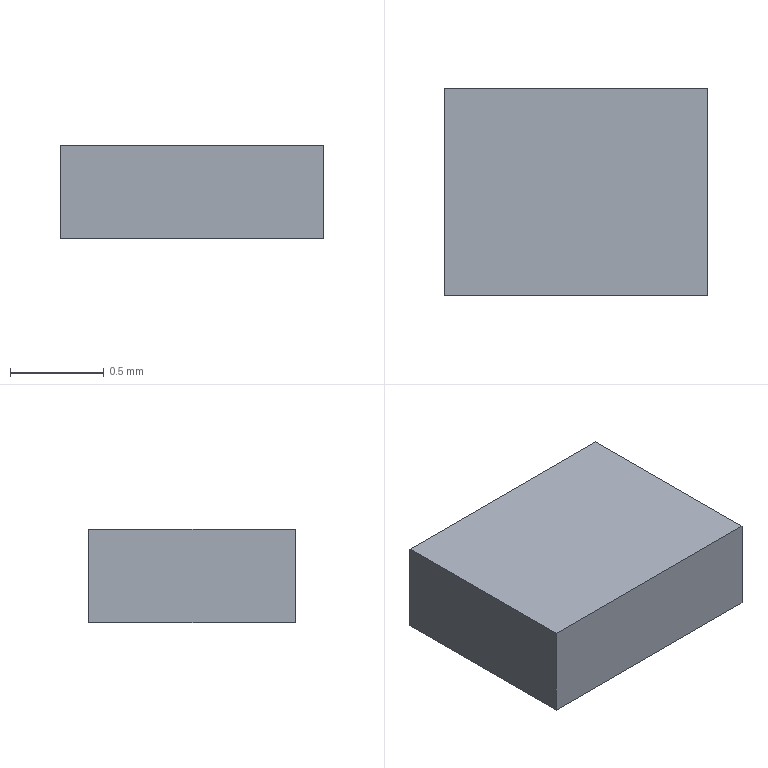Part | Creo | 1 solid | 6 faces | box 1.4 x 1.1 x 0.5001 mm | volume 0.7702 mm3 | plane 6
STEP:
#1=CARTESIAN_POINT('',(0.,0.,0.));
#2=DIRECTION('',(0.,0.,1.));
#3=DIRECTION('',(1.,0.,0.));
#4=AXIS2_PLACEMENT_3D('',#1,#2,#3);
#5=CARTESIAN_POINT('',(-0.7,0.55,0.));
#6=VERTEX_POINT('',#5);
#7=CARTESIAN_POINT('',(-0.7,-0.55,0.));
#8=VERTEX_POINT('',#7);
#9=CARTESIAN_POINT('',(-0.7,0.55,0.));
#10=DIRECTION('',(0.,-1.,0.));
#11=VECTOR('',#10,1.1);
#12=LINE('',#9,#11);
#13=EDGE_CURVE('',#6,#8,#12,.T.);
#14=ORIENTED_EDGE('',*,*,#13,.T.);
#15=CARTESIAN_POINT('',(0.7,-0.55,0.));
#16=VERTEX_POINT('',#15);
#17=CARTESIAN_POINT('',(-0.7,-0.55,0.));
#18=DIRECTION('',(1.,0.,0.));
#19=VECTOR('',#18,1.4);
#20=LINE('',#17,#19);
#21=EDGE_CURVE('',#8,#16,#20,.T.);
#22=ORIENTED_EDGE('',*,*,#21,.T.);
#23=CARTESIAN_POINT('',(0.7,0.55,0.));
#24=VERTEX_POINT('',#23);
#25=CARTESIAN_POINT('',(0.7,-0.55,0.));
#26=DIRECTION('',(0.,1.,0.));
#27=VECTOR('',#26,1.1);
#28=LINE('',#25,#27);
#29=EDGE_CURVE('',#16,#24,#28,.T.);
#30=ORIENTED_EDGE('',*,*,#29,.T.);
#31=CARTESIAN_POINT('',(0.7,0.55,0.));
#32=DIRECTION('',(-1.,0.,0.));
#33=VECTOR('',#32,1.4);
#34=LINE('',#31,#33);
#35=EDGE_CURVE('',#24,#6,#34,.T.);
#36=ORIENTED_EDGE('',*,*,#35,.T.);
#37=EDGE_LOOP('',(#14,#22,#30,#36));
#38=FACE_OUTER_BOUND('',#37,.F.);
#39=CARTESIAN_POINT('',(0.,0.,0.));
#40=DIRECTION('',(0.,0.,1.));
#41=DIRECTION('',(1.,0.,0.));
#42=AXIS2_PLACEMENT_3D('',#39,#40,#41);
#43=PLANE('',#42);
#44=ADVANCED_FACE('',(#38),#43,.F.);
#45=ORIENTED_EDGE('',*,*,#13,.F.);
#46=CARTESIAN_POINT('',(-0.7,0.55,0.5001));
#47=VERTEX_POINT('',#46);
#48=CARTESIAN_POINT('',(-0.7,0.55,0.));
#49=DIRECTION('',(0.,0.,1.));
#50=VECTOR('',#49,0.5001);
#51=LINE('',#48,#50);
#52=EDGE_CURVE('',#6,#47,#51,.T.);
#53=ORIENTED_EDGE('',*,*,#52,.T.);
#54=CARTESIAN_POINT('',(-0.7,-0.55,0.5001));
#55=VERTEX_POINT('',#54);
#56=CARTESIAN_POINT('',(-0.7,0.55,0.5001));
#57=DIRECTION('',(0.,-1.,0.));
#58=VECTOR('',#57,1.1);
#59=LINE('',#56,#58);
#60=EDGE_CURVE('',#47,#55,#59,.T.);
#61=ORIENTED_EDGE('',*,*,#60,.T.);
#62=CARTESIAN_POINT('',(-0.7,-0.55,0.));
#63=DIRECTION('',(0.,0.,1.));
#64=VECTOR('',#63,0.5001);
#65=LINE('',#62,#64);
#66=EDGE_CURVE('',#8,#55,#65,.T.);
#67=ORIENTED_EDGE('',*,*,#66,.F.);
#68=EDGE_LOOP('',(#45,#53,#61,#67));
#69=FACE_OUTER_BOUND('',#68,.F.);
#70=CARTESIAN_POINT('',(-0.7,0.55,0.));
#71=DIRECTION('',(-1.,0.,0.));
#72=DIRECTION('',(0.,-1.,0.));
#73=AXIS2_PLACEMENT_3D('',#70,#71,#72);
#74=PLANE('',#73);
#75=ADVANCED_FACE('',(#69),#74,.T.);
#76=ORIENTED_EDGE('',*,*,#35,.F.);
#77=CARTESIAN_POINT('',(0.7,0.55,0.5001));
#78=VERTEX_POINT('',#77);
#79=CARTESIAN_POINT('',(0.7,0.55,0.));
#80=DIRECTION('',(0.,0.,1.));
#81=VECTOR('',#80,0.5001);
#82=LINE('',#79,#81);
#83=EDGE_CURVE('',#24,#78,#82,.T.);
#84=ORIENTED_EDGE('',*,*,#83,.T.);
#85=CARTESIAN_POINT('',(0.7,0.55,0.5001));
#86=DIRECTION('',(-1.,0.,0.));
#87=VECTOR('',#86,1.4);
#88=LINE('',#85,#87);
#89=EDGE_CURVE('',#78,#47,#88,.T.);
#90=ORIENTED_EDGE('',*,*,#89,.T.);
#91=ORIENTED_EDGE('',*,*,#52,.F.);
#92=EDGE_LOOP('',(#76,#84,#90,#91));
#93=FACE_OUTER_BOUND('',#92,.F.);
#94=CARTESIAN_POINT('',(0.7,0.55,0.));
#95=DIRECTION('',(0.,1.,0.));
#96=DIRECTION('',(-1.,0.,0.));
#97=AXIS2_PLACEMENT_3D('',#94,#95,#96);
#98=PLANE('',#97);
#99=ADVANCED_FACE('',(#93),#98,.T.);
#100=ORIENTED_EDGE('',*,*,#29,.F.);
#101=CARTESIAN_POINT('',(0.7,-0.55,0.5001));
#102=VERTEX_POINT('',#101);
#103=CARTESIAN_POINT('',(0.7,-0.55,0.));
#104=DIRECTION('',(0.,0.,1.));
#105=VECTOR('',#104,0.5001);
#106=LINE('',#103,#105);
#107=EDGE_CURVE('',#16,#102,#106,.T.);
#108=ORIENTED_EDGE('',*,*,#107,.T.);
#109=CARTESIAN_POINT('',(0.7,-0.55,0.5001));
#110=DIRECTION('',(0.,1.,0.));
#111=VECTOR('',#110,1.1);
#112=LINE('',#109,#111);
#113=EDGE_CURVE('',#102,#78,#112,.T.);
#114=ORIENTED_EDGE('',*,*,#113,.T.);
#115=ORIENTED_EDGE('',*,*,#83,.F.);
#116=EDGE_LOOP('',(#100,#108,#114,#115));
#117=FACE_OUTER_BOUND('',#116,.F.);
#118=CARTESIAN_POINT('',(0.7,-0.55,0.));
#119=DIRECTION('',(1.,0.,0.));
#120=DIRECTION('',(0.,1.,0.));
#121=AXIS2_PLACEMENT_3D('',#118,#119,#120);
#122=PLANE('',#121);
#123=ADVANCED_FACE('',(#117),#122,.T.);
#124=ORIENTED_EDGE('',*,*,#21,.F.);
#125=ORIENTED_EDGE('',*,*,#66,.T.);
#126=CARTESIAN_POINT('',(-0.7,-0.55,0.5001));
#127=DIRECTION('',(1.,0.,0.));
#128=VECTOR('',#127,1.4);
#129=LINE('',#126,#128);
#130=EDGE_CURVE('',#55,#102,#129,.T.);
#131=ORIENTED_EDGE('',*,*,#130,.T.);
#132=ORIENTED_EDGE('',*,*,#107,.F.);
#133=EDGE_LOOP('',(#124,#125,#131,#132));
#134=FACE_OUTER_BOUND('',#133,.F.);
#135=CARTESIAN_POINT('',(-0.7,-0.55,0.));
#136=DIRECTION('',(0.,-1.,0.));
#137=DIRECTION('',(1.,0.,0.));
#138=AXIS2_PLACEMENT_3D('',#135,#136,#137);
#139=PLANE('',#138);
#140=ADVANCED_FACE('',(#134),#139,.T.);
#141=ORIENTED_EDGE('',*,*,#60,.F.);
#142=ORIENTED_EDGE('',*,*,#89,.F.);
#143=ORIENTED_EDGE('',*,*,#113,.F.);
#144=ORIENTED_EDGE('',*,*,#130,.F.);
#145=EDGE_LOOP('',(#141,#142,#143,#144));
#146=FACE_OUTER_BOUND('',#145,.F.);
#147=CARTESIAN_POINT('',(0.,0.,0.5001));
#148=DIRECTION('',(0.,0.,1.));
#149=DIRECTION('',(1.,0.,0.));
#150=AXIS2_PLACEMENT_3D('',#147,#148,#149);
#151=PLANE('',#150);
#152=ADVANCED_FACE('',(#146),#151,.T.);
#153=CLOSED_SHELL('',(#44,#75,#99,#123,#140,#152));
#154=MANIFOLD_SOLID_BREP('',#153);
#155=(LENGTH_UNIT()NAMED_UNIT(*)SI_UNIT(.MILLI.,.METRE.));
#156=UNCERTAINTY_MEASURE_WITH_UNIT(LENGTH_MEASURE(0.0001849),#155,'','');
#157=(NAMED_UNIT(*)PLANE_ANGLE_UNIT()SI_UNIT($,.RADIAN.));
#158=PLANE_ANGLE_MEASURE_WITH_UNIT(PLANE_ANGLE_MEASURE(0.01745),#157);
#159=(CONVERSION_BASED_UNIT('DEGREE',#158)NAMED_UNIT(*)PLANE_ANGLE_UNIT());
#160=(NAMED_UNIT(*)SI_UNIT($,.STERADIAN.)SOLID_ANGLE_UNIT());
#161=(GEOMETRIC_REPRESENTATION_CONTEXT(3)GLOBAL_UNCERTAINTY_ASSIGNED_CONTEXT((#156))GLOBAL_UNIT_ASSIGNED_CONTEXT((#155,#159,#160))REPRESENTATION_CONTEXT('',''));
#162=ADVANCED_BREP_SHAPE_REPRESENTATION('',(#4,#154),#161);